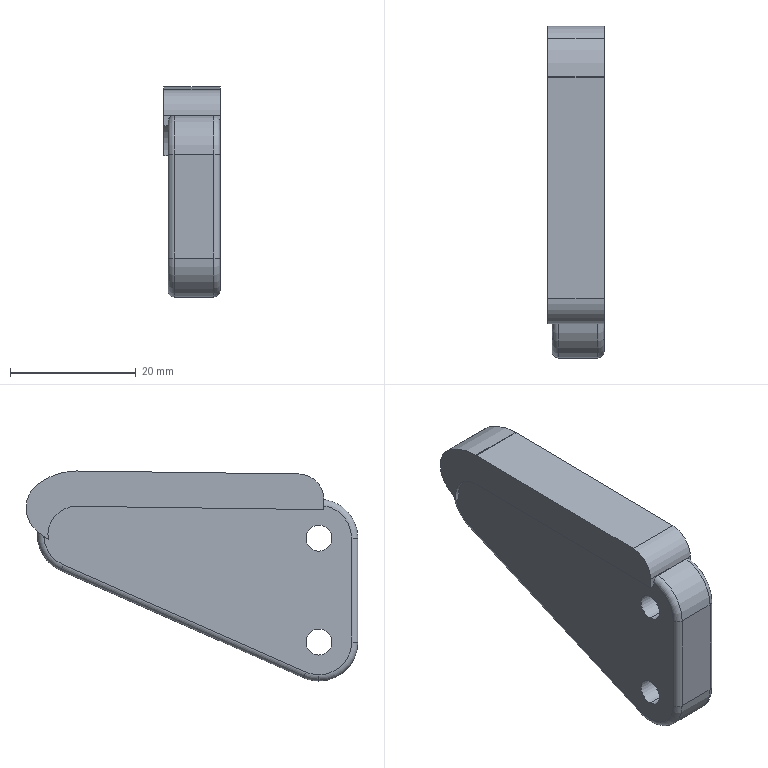Part | SolidWorks | features ICE 5, CirPattern 1, Extrusion 1, Fillet 1, LPattern 1, Scale 1 | 1 solid | 97 faces | box 8.915 x 52.717 x 33.373 mm | volume 8638 mm3 | plane 65 | cylinder 24 | torus 8 | commonest cylinder face diameters 12.383 x7 1.981 x4 4.127 x2 4.128 x2 18.987 x2 20.307 x2